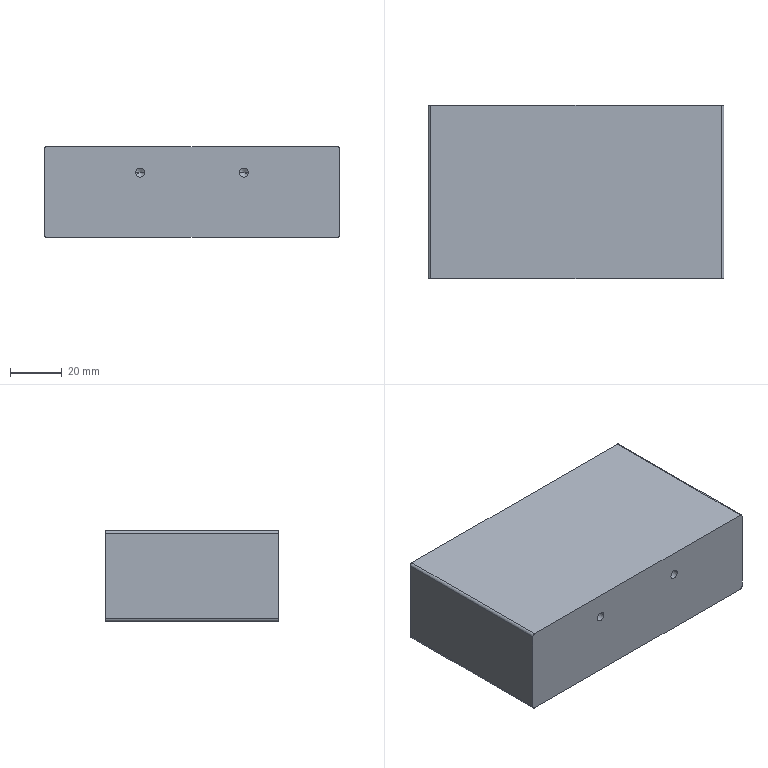NC program | NX | posted with a generic post | part box 114 x 67 x 35 mm
Whole program:
N10 G17 G21 G94 G90
(FLOOR_WALL , TOOL : D63)
N12 T01 M6
N14 G54
N16 G17 G0 G90 X-94.5 Y36.497 B0. C0. S6500 M3
N18 G43 Z30. H1
N20 Z3.
N22 G94 G1 Z0. F1250.
N24 X-91.5
N26 X91.5
N28 Y12.599
N30 X-91.5
N32 Y-11.3
N34 X91.5
N36 X94.5
N38 Z3.
N40 G0 Z30.
N42 M5
(ZLEVEL_PROFILE , TOOL : D10)
N44 T09 M6
N46 G54
N48 G17 G0 G90 X-47.703 Y38.6 B0. C0. S9500 M3
N50 G43 Z30. H9
N52 Z1.5
N54 G94 G1 X0. Z-1. F1000.
N56 X57. F3000.
N58 G2 X62.1 Y33.5 R5.1
N60 G1 Y-33.5
N62 G2 X57. Y-38.6 R5.1
N64 G1 X-57.
N66 G2 X-62.1 Y-33.5 R5.1
N68 G1 Y33.5
N70 G2 X-57. Y38.6 R5.1
N72 G1 X0.
N74 X56.516 Z-1.986
N76 X56.903 Z-1.993
N78 X57.29 Y38.592 Z-2.
N80 G2 X62.1 Y33.5 R5.1
N82 G1 Y-33.5
N84 G2 X57. Y-38.6 R5.1
N86 G1 X-57.
N88 G2 X-62.1 Y-33.5 R5.1
N90 G1 Y33.5
N92 G2 X-57. Y38.6 R5.1
N94 G1 X0.
N96 X56.516 Z-2.986
N98 X56.903 Z-2.993
N100 X57.29 Y38.592 Z-3.
N102 G2 X62.1 Y33.5 R5.1
N104 G1 Y-33.5
N106 G2 X57. Y-38.6 R5.1
N108 G1 X-57.
N110 G2 X-62.1 Y-33.5 R5.1
N112 G1 Y33.5
N114 G2 X-57. Y38.6 R5.1
N116 G1 X0.
N118 X56.516 Z-3.986
N120 X56.903 Z-3.993
N122 X57.29 Y38.592 Z-4.
N124 G2 X62.1 Y33.5 R5.1
N126 G1 Y-33.5
N128 G2 X57. Y-38.6 R5.1
N130 G1 X-57.
N132 G2 X-62.1 Y-33.5 R5.1
N134 G1 Y33.5
N136 G2 X-57. Y38.6 R5.1
N138 G1 X0.
N140 X56.516 Z-4.986
N142 X56.903 Z-4.993
N144 X57.29 Y38.592 Z-5.
N146 G2 X62.1 Y33.5 R5.1
N148 G1 Y-33.5
N150 G2 X57. Y-38.6 R5.1
N152 G1 X-57.
N154 G2 X-62.1 Y-33.5 R5.1
N156 G1 Y33.5
N158 G2 X-57. Y38.6 R5.1
N160 G1 X0.
N162 X56.516 Z-5.986
N164 X56.903 Z-5.993
N166 X57.29 Y38.592 Z-6.
N168 G2 X62.1 Y33.5 R5.1
N170 G1 Y-33.5
N172 G2 X57. Y-38.6 R5.1
N174 G1 X-57.
N176 G2 X-62.1 Y-33.5 R5.1
N178 G1 Y33.5
N180 G2 X-57. Y38.6 R5.1
N182 G1 X0.
N184 X56.516 Z-6.986
N186 X56.903 Z-6.993
N188 X57.29 Y38.592 Z-7.
N190 G2 X62.1 Y33.5 R5.1
N192 G1 Y-33.5
N194 G2 X57. Y-38.6 R5.1
N196 G1 X-57.
N198 G2 X-62.1 Y-33.5 R5.1
N200 G1 Y33.5
N202 G2 X-57. Y38.6 R5.1
N204 G1 X0.
N206 X56.516 Z-7.986
N208 X56.903 Z-7.993
N210 X57.29 Y38.592 Z-8.
N212 G2 X62.1 Y33.5 R5.1
N214 G1 Y-33.5
N216 G2 X57. Y-38.6 R5.1
N218 G1 X-57.
N220 G2 X-62.1 Y-33.5 R5.1
N222 G1 Y33.5
N224 G2 X-57. Y38.6 R5.1
N226 G1 X0.
N228 X56.516 Z-8.986
N230 X56.903 Z-8.993
N232 X57.29 Y38.592 Z-9.
N234 G2 X62.1 Y33.5 R5.1
N236 G1 Y-33.5
N238 G2 X57. Y-38.6 R5.1
N240 G1 X-57.
N242 G2 X-62.1 Y-33.5 R5.1
N244 G1 Y33.5
N246 G2 X-57. Y38.6 R5.1
N248 G1 X0.
N250 X56.516 Z-9.986
N252 X56.903 Z-9.993
N254 X57.29 Y38.592 Z-10.
N256 G2 X62.1 Y33.5 R5.1
N258 G1 Y-33.5
N260 G2 X57. Y-38.6 R5.1
N262 G1 X-57.
N264 G2 X-62.1 Y-33.5 R5.1
N266 G1 Y33.5
N268 G2 X-57. Y38.6 R5.1
N270 G1 X0.
N272 X56.516 Z-10.986
N274 X56.903 Z-10.993
N276 X57.29 Y38.592 Z-11.
N278 G2 X62.1 Y33.5 R5.1
N280 G1 Y-33.5
N282 G2 X57. Y-38.6 R5.1
N284 G1 X-57.
N286 G2 X-62.1 Y-33.5 R5.1
N288 G1 Y33.5
N290 G2 X-57. Y38.6 R5.1
N292 G1 X0.
N294 X56.516 Z-11.986
N296 X56.903 Z-11.993
N298 X57.29 Y38.592 Z-12.
N300 G2 X62.1 Y33.5 R5.1
N302 G1 Y-33.5
N304 G2 X57. Y-38.6 R5.1
N306 G1 X-57.
N308 G2 X-62.1 Y-33.5 R5.1
N310 G1 Y33.5
N312 G2 X-57. Y38.6 R5.1
N314 G1 X0.
N316 X56.516 Z-12.986
N318 X56.903 Z-12.993
N320 X57.29 Y38.592 Z-13.
N322 G2 X62.1 Y33.5 R5.1
N324 G1 Y-33.5
N326 G2 X57. Y-38.6 R5.1
N328 G1 X-57.
N330 G2 X-62.1 Y-33.5 R5.1
N332 G1 Y33.5
N334 G2 X-57. Y38.6 R5.1
N336 G1 X0.
N338 X56.516 Z-13.986
N340 X56.903 Z-13.993
N342 X57.29 Y38.592 Z-14.
N344 G2 X62.1 Y33.5 R5.1
N346 G1 Y-33.5
N348 G2 X57. Y-38.6 R5.1
N350 G1 X-57.
N352 G2 X-62.1 Y-33.5 R5.1
N354 G1 Y33.5
N356 G2 X-57. Y38.6 R5.1
N358 G1 X0.
N360 X56.516 Z-14.986
N362 X56.903 Z-14.993
N364 X57.29 Y38.592 Z-15.
N366 G2 X62.1 Y33.5 R5.1
N368 G1 Y-33.5
N370 G2 X57. Y-38.6 R5.1
N372 G1 X-57.
N374 G2 X-62.1 Y-33.5 R5.1
N376 G1 Y33.5
N378 G2 X-57. Y38.6 R5.1
N380 G1 X0.
N382 X56.516 Z-15.986
N384 X56.903 Z-15.993
N386 X57.29 Y38.592 Z-16.
N388 G2 X62.1 Y33.5 R5.1
N390 G1 Y-33.5
N392 G2 X57. Y-38.6 R5.1
N394 G1 X-57.
N396 G2 X-62.1 Y-33.5 R5.1
N398 G1 Y33.5
N400 G2 X-57. Y38.6 R5.1
N402 G1 X0.
N404 X56.516 Z-16.986
N406 X56.903 Z-16.993
N408 X57.29 Y38.592 Z-17.
N410 G2 X62.1 Y33.5 R5.1
N412 G1 Y-33.5
N414 G2 X57. Y-38.6 R5.1
N416 G1 X-57.
N418 G2 X-62.1 Y-33.5 R5.1
N420 G1 Y33.5
N422 G2 X-57. Y38.6 R5.1
N424 G1 X0.
N426 X56.516 Z-17.986
N428 X56.903 Z-17.993
N430 X57.29 Y38.592 Z-18.
N432 G2 X62.1 Y33.5 R5.1
N434 G1 Y-33.5
N436 G2 X57. Y-38.6 R5.1
N438 G1 X-57.
N440 G2 X-62.1 Y-33.5 R5.1
N442 G1 Y33.5
N444 G2 X-57. Y38.6 R5.1
N446 G1 X0.
N448 X56.516 Z-18.986
N450 X56.903 Z-18.993
N452 X57.29 Y38.592 Z-19.
N454 G2 X62.1 Y33.5 R5.1
N456 G1 Y-33.5
N458 G2 X57. Y-38.6 R5.1
N460 G1 X-57.
N462 G2 X-62.1 Y-33.5 R5.1
N464 G1 Y33.5
N466 G2 X-57. Y38.6 R5.1
N468 G1 X0.
N470 X56.516 Z-19.986
N472 X56.903 Z-19.993
N474 X57.29 Y38.592 Z-20.
N476 G2 X62.1 Y33.5 R5.1
N478 G1 Y-33.5
N480 G2 X57. Y-38.6 R5.1
N482 G1 X-57.
N484 G2 X-62.1 Y-33.5 R5.1
N486 G1 Y33.5
N488 G2 X-57. Y38.6 R5.1
N490 G1 X0.
N492 X56.516 Z-20.986
N494 X56.903 Z-20.993
N496 X57.29 Y38.592 Z-21.
N498 G2 X62.1 Y33.5 R5.1
N500 G1 Y-33.5
N502 G2 X57. Y-38.6 R5.1
N504 G1 X-57.
N506 G2 X-62.1 Y-33.5 R5.1
N508 G1 Y33.5
N510 G2 X-57. Y38.6 R5.1
N512 G1 X0.
N514 X56.516 Z-21.986
N516 X56.903 Z-21.993
N518 X57.29 Y38.592 Z-22.
N520 G2 X62.1 Y33.5 R5.1
N522 G1 Y-33.5
N524 G2 X57. Y-38.6 R5.1
N526 G1 X-57.
N528 G2 X-62.1 Y-33.5 R5.1
N530 G1 Y33.5
N532 G2 X-57. Y38.6 R5.1
N534 G1 X0.
N536 X56.516 Z-22.986
N538 X56.903 Z-22.993
N540 X57.29 Y38.592 Z-23.
N542 G2 X62.1 Y33.5 R5.1
N544 G1 Y-33.5
N546 G2 X57. Y-38.6 R5.1
N548 G1 X-57.
N550 G2 X-62.1 Y-33.5 R5.1
N552 G1 Y33.5
N554 G2 X-57. Y38.6 R5.1
N556 G1 X0.
N558 X56.516 Z-23.986
N560 X56.903 Z-23.993
N562 X57.29 Y38.592 Z-24.
N564 G2 X62.1 Y33.5 R5.1
N566 G1 Y-33.5
N568 G2 X57. Y-38.6 R5.1
N570 G1 X-57.
N572 G2 X-62.1 Y-33.5 R5.1
N574 G1 Y33.5
N576 G2 X-57. Y38.6 R5.1
N578 G1 X0.
N580 X56.516 Z-24.986
N582 X56.903 Z-24.993
N584 X57.29 Y38.592 Z-25.
N586 G2 X62.1 Y33.5 R5.1
N588 G1 Y-33.5
N590 G2 X57. Y-38.6 R5.1
N592 G1 X-57.
N594 G2 X-62.1 Y-33.5 R5.1
N596 G1 Y33.5
N598 G2 X-57. Y38.6 R5.1
N600 G1 X0.
N602 X56.516 Z-25.986
N604 X56.903 Z-25.993
N606 X57.29 Y38.592 Z-26.
N608 G2 X62.1 Y33.5 R5.1
N610 G1 Y-33.5
N612 G2 X57. Y-38.6 R5.1
N614 G1 X-57.
N616 G2 X-62.1 Y-33.5 R5.1
N618 G1 Y33.5
N620 G2 X-57. Y38.6 R5.1
N622 G1 X0.
N624 X56.516 Z-26.986
N626 X56.903 Z-26.993
N628 X57.29 Y38.592 Z-27.
N630 G2 X62.1 Y33.5 R5.1
N632 G1 Y-33.5
N634 G2 X57. Y-38.6 R5.1
N636 G1 X-57.
N638 G2 X-62.1 Y-33.5 R5.1
N640 G1 Y33.5
N642 G2 X-57. Y38.6 R5.1
N644 G1 X0.
N646 X56.516 Z-27.986
N648 X56.903 Z-27.993
N650 X57.29 Y38.592 Z-28.
N652 G2 X62.1 Y33.5 R5.1
N654 G1 Y-33.5
N656 G2 X57. Y-38.6 R5.1
N658 G1 X-57.
N660 G2 X-62.1 Y-33.5 R5.1
N662 G1 Y33.5
N664 G2 X-57. Y38.6 R5.1
N666 G1 X0.
N668 X56.516 Z-28.986
N670 X56.903 Z-28.993
N672 X57.29 Y38.592 Z-29.
N674 G2 X62.1 Y33.5 R5.1
N676 G1 Y-33.5
N678 G2 X57. Y-38.6 R5.1
N680 G1 X-57.
N682 G2 X-62.1 Y-33.5 R5.1
N684 G1 Y33.5
N686 G2 X-57. Y38.6 R5.1
N688 G1 X0.
N690 X56.516 Z-29.986
N692 X56.903 Z-29.993
N694 X57.29 Y38.592 Z-30.
N696 G2 X62.1 Y33.5 R5.1
N698 G1 Y-33.5
N700 G2 X57. Y-38.6 R5.1
N702 G1 X-57.
N704 G2 X-62.1 Y-33.5 R5.1
N706 G1 Y33.5
N708 G2 X-57. Y38.6 R5.1
N710 G1 X0.
N712 X56.516 Z-30.986
N714 X56.903 Z-30.993
N716 X57.29 Y38.592 Z-31.
N718 G2 X62.1 Y33.5 R5.1
N720 G1 Y-33.5
N722 G2 X57. Y-38.6 R5.1
N724 G1 X-57.
N726 G2 X-62.1 Y-33.5 R5.1
N728 G1 Y33.5
N730 G2 X-57. Y38.6 R5.1
N732 G1 X0.
N734 X56.516 Z-31.986
N736 X56.903 Z-31.993
N738 X57.29 Y38.592 Z-32.
N740 G2 X62.1 Y33.5 R5.1
N742 G1 Y-33.5
N744 G2 X57. Y-38.6 R5.1
N746 G1 X-57.
N748 G2 X-62.1 Y-33.5 R5.1
N750 G1 Y33.5
N752 G2 X-57. Y38.6 R5.1
N754 G1 X0.
N756 X56.516 Z-32.986
N758 X56.903 Z-32.993
N760 X57.29 Y38.592 Z-33.
N762 G2 X62.1 Y33.5 R5.1
N764 G1 Y-33.5
N766 G2 X57. Y-38.6 R5.1
N768 G1 X-57.
N770 G2 X-62.1 Y-33.5 R5.1
N772 G1 Y33.5
N774 G2 X-57. Y38.6 R5.1
N776 G1 X0.
N778 X56.516 Z-33.986
N780 X56.903 Z-33.993
N782 X57.29 Y38.592 Z-34.
N784 G2 X62.1 Y33.5 R5.1
N786 G1 Y-33.5
N788 G2 X57. Y-38.6 R5.1
N790 G1 X-57.
N792 G2 X-62.1 Y-33.5 R5.1
N794 G1 Y33.5
N796 G2 X-57. Y38.6 R5.1
N798 G1 X0.
N800 X56.516 Z-34.986
N802 X56.903 Z-34.993
N804 X57.29 Y38.592 Z-35.
N806 G2 X62.1 Y33.5 R5.1
N808 G1 Y-33.5
N810 G2 X57. Y-38.6 R5.1
N812 G1 X-57.
N814 G2 X-62.1 Y-33.5 R5.1
N816 G1 Y33.5
N818 G2 X-57. Y38.6 R5.1
N820 G1 X57.
N822 G2 X57.29 Y38.592 R5.1
N824 G1 Z-33.5
N826 G0 Z30.
N828 M5
(ZLEVEL_PROFILE_COPY_COPY , TOOL : D10JING)
N830 T10 M6
N832 G54
N834 G17 G0 G90 X-58.622 Y40.309 B0. C0. S9500 M3
N836 G43 Z30. H10
N838 Z-16.
N840 G94 G1 Z-17.5 F1000.
N842 X-57.866 Y39.
N844 G3 X-57. Y38.5 R1.
N846 G1 X57. F1200.
N848 G2 X62. Y33.5 R5.
N850 G1 Y-33.5
N852 G2 X57. Y-38.5 R5.
N854 G1 X-57.
N856 G2 X-62. Y-33.5 R5.
N858 G1 Y33.5
N860 G2 X-57. Y38.5 R5.
N862 G3 X-56.134 Y39. R1.
N864 G1 X-55.268 Y40.5
N866 Z-16.
N868 G0 Z30.
N870 X-58.622 Y40.309
N872 Z-33.5
N874 G1 Z-35. F1000.
N876 X-57.866 Y39.
N878 G3 X-57. Y38.5 R1.
N880 G1 X57. F1200.
N882 G2 X62. Y33.5 R5.
N884 G1 Y-33.5
N886 G2 X57. Y-38.5 R5.
N888 G1 X-57.
N890 G2 X-62. Y-33.5 R5.
N892 G1 Y33.5
N894 G2 X-57. Y38.5 R5.
N896 G3 X-56.134 Y39. R1.
N898 G1 X-55.268 Y40.5
N900 Z-33.5
N902 G0 Z30.
N904 M5
N906 M2